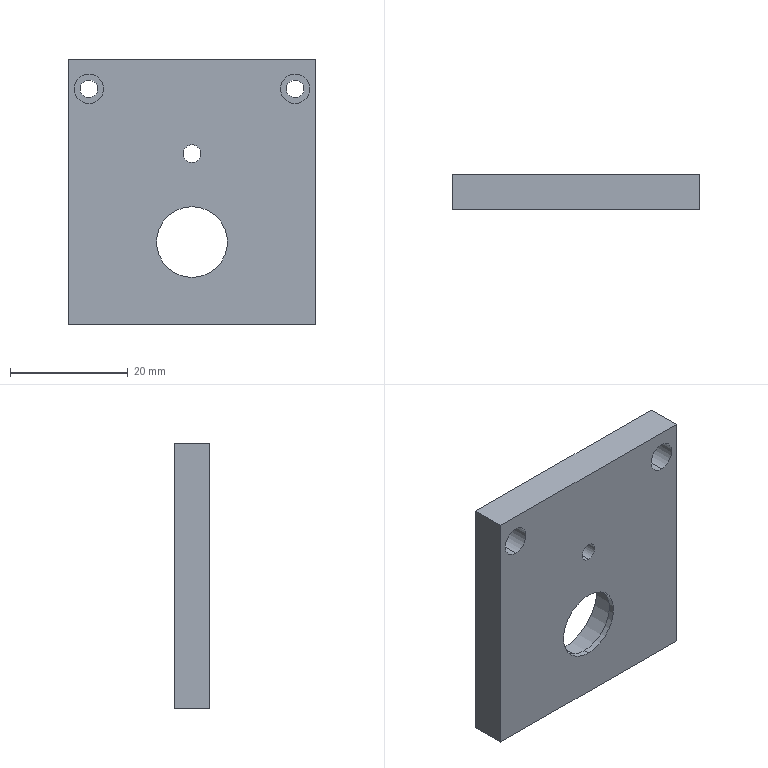Part | SolidWorks | features ICE 3, Cut 1, Extrusion 1, HoleWzd 1 | 1 solid | 31 faces | box 42 x 6 x 45 mm | volume 9918 mm3 | cylinder 18 | plane 9 | cone 4 | commonest cylinder face diameters 3 x6 2.5 x4 5 x4 12 x2 16 x2
STEP:
#1=CARTESIAN_POINT('',(13.5,3.,-5.25));
#2=VERTEX_POINT('',#1);
#3=CARTESIAN_POINT('',(13.5,3.,-7.75));
#4=VERTEX_POINT('',#3);
#5=CARTESIAN_POINT('',(13.5,3.,-6.5));
#6=DIRECTION('',(1.,0.,0.));
#7=DIRECTION('',(0.,0.,-1.));
#8=AXIS2_PLACEMENT_3D('',#5,#6,#7);
#9=CIRCLE('',#8,1.25);
#10=EDGE_CURVE('',#2,#4,#9,.T.);
#11=ORIENTED_EDGE('',*,*,#10,.F.);
#12=CARTESIAN_POINT('',(21.,3.,-5.25));
#13=VERTEX_POINT('',#12);
#14=CARTESIAN_POINT('',(21.,3.,-5.25));
#15=DIRECTION('',(1.,0.,0.));
#16=VECTOR('',#15,1000.);
#17=LINE('',#14,#16);
#18=EDGE_CURVE('',#2,#13,#17,.T.);
#19=ORIENTED_EDGE('',*,*,#18,.T.);
#20=CARTESIAN_POINT('',(21.,3.,-7.75));
#21=VERTEX_POINT('',#20);
#22=CARTESIAN_POINT('',(21.,3.,-6.5));
#23=DIRECTION('',(1.,0.,0.));
#24=DIRECTION('',(0.,0.,-1.));
#25=AXIS2_PLACEMENT_3D('',#22,#23,#24);
#26=CIRCLE('',#25,1.25);
#27=EDGE_CURVE('',#13,#21,#26,.T.);
#28=ORIENTED_EDGE('',*,*,#27,.T.);
#29=CARTESIAN_POINT('',(21.,3.,-7.75));
#30=DIRECTION('',(1.,0.,0.));
#31=VECTOR('',#30,1000.);
#32=LINE('',#29,#31);
#33=EDGE_CURVE('',#4,#21,#32,.T.);
#34=ORIENTED_EDGE('',*,*,#33,.F.);
#35=EDGE_LOOP('',(#11,#19,#28,#34));
#36=FACE_OUTER_BOUND('',#35,.T.);
#37=CARTESIAN_POINT('',(21.,3.,-6.5));
#38=DIRECTION('',(1.,0.,0.));
#39=DIRECTION('',(0.,0.,-1.));
#40=AXIS2_PLACEMENT_3D('',#37,#38,#39);
#41=CYLINDRICAL_SURFACE('',#40,1.25);
#42=ADVANCED_FACE('',(#36),#41,.F.);
#43=CARTESIAN_POINT('',(12.749,3.,-6.5));
#44=VERTEX_POINT('',#43);
#45=CARTESIAN_POINT('',(13.5,3.,-7.75));
#46=DIRECTION('',(0.515,0.,-0.8572));
#47=VECTOR('',#46,1000.);
#48=LINE('',#45,#47);
#49=EDGE_CURVE('',#44,#4,#48,.T.);
#50=ORIENTED_EDGE('',*,*,#49,.F.);
#51=CARTESIAN_POINT('',(13.5,3.,-5.25));
#52=DIRECTION('',(0.515,0.,0.8572));
#53=VECTOR('',#52,1000.);
#54=LINE('',#51,#53);
#55=EDGE_CURVE('',#44,#2,#54,.T.);
#56=ORIENTED_EDGE('',*,*,#55,.T.);
#57=ORIENTED_EDGE('',*,*,#10,.T.);
#58=EDGE_LOOP('',(#50,#56,#57));
#59=FACE_OUTER_BOUND('',#58,.T.);
#60=CARTESIAN_POINT('',(13.5,3.,-6.5));
#61=DIRECTION('',(1.,0.,0.));
#62=DIRECTION('',(0.,0.,-1.));
#63=AXIS2_PLACEMENT_3D('',#60,#61,#62);
#64=CONICAL_SURFACE('',#63,1.25,1.03);
#65=ADVANCED_FACE('',(#59),#64,.F.);
#66=CARTESIAN_POINT('',(13.5,3.,4.25));
#67=VERTEX_POINT('',#66);
#68=CARTESIAN_POINT('',(13.5,3.,1.75));
#69=VERTEX_POINT('',#68);
#70=CARTESIAN_POINT('',(13.5,3.,3.));
#71=DIRECTION('',(1.,0.,0.));
#72=DIRECTION('',(0.,0.,-1.));
#73=AXIS2_PLACEMENT_3D('',#70,#71,#72);
#74=CIRCLE('',#73,1.25);
#75=EDGE_CURVE('',#67,#69,#74,.T.);
#76=ORIENTED_EDGE('',*,*,#75,.F.);
#77=CARTESIAN_POINT('',(21.,3.,4.25));
#78=VERTEX_POINT('',#77);
#79=CARTESIAN_POINT('',(21.,3.,4.25));
#80=DIRECTION('',(1.,0.,0.));
#81=VECTOR('',#80,1000.);
#82=LINE('',#79,#81);
#83=EDGE_CURVE('',#67,#78,#82,.T.);
#84=ORIENTED_EDGE('',*,*,#83,.T.);
#85=CARTESIAN_POINT('',(21.,3.,1.75));
#86=VERTEX_POINT('',#85);
#87=CARTESIAN_POINT('',(21.,3.,3.));
#88=DIRECTION('',(1.,0.,0.));
#89=DIRECTION('',(0.,0.,-1.));
#90=AXIS2_PLACEMENT_3D('',#87,#88,#89);
#91=CIRCLE('',#90,1.25);
#92=EDGE_CURVE('',#78,#86,#91,.T.);
#93=ORIENTED_EDGE('',*,*,#92,.T.);
#94=CARTESIAN_POINT('',(21.,3.,1.75));
#95=DIRECTION('',(1.,0.,0.));
#96=VECTOR('',#95,1000.);
#97=LINE('',#94,#96);
#98=EDGE_CURVE('',#69,#86,#97,.T.);
#99=ORIENTED_EDGE('',*,*,#98,.F.);
#100=EDGE_LOOP('',(#76,#84,#93,#99));
#101=FACE_OUTER_BOUND('',#100,.T.);
#102=CARTESIAN_POINT('',(21.,3.,3.));
#103=DIRECTION('',(1.,0.,0.));
#104=DIRECTION('',(0.,0.,-1.));
#105=AXIS2_PLACEMENT_3D('',#102,#103,#104);
#106=CYLINDRICAL_SURFACE('',#105,1.25);
#107=ADVANCED_FACE('',(#101),#106,.F.);
#108=CARTESIAN_POINT('',(12.749,3.,3.));
#109=VERTEX_POINT('',#108);
#110=CARTESIAN_POINT('',(13.5,3.,1.75));
#111=DIRECTION('',(0.515,0.,-0.8572));
#112=VECTOR('',#111,1000.);
#113=LINE('',#110,#112);
#114=EDGE_CURVE('',#109,#69,#113,.T.);
#115=ORIENTED_EDGE('',*,*,#114,.F.);
#116=CARTESIAN_POINT('',(13.5,3.,4.25));
#117=DIRECTION('',(0.515,0.,0.8572));
#118=VECTOR('',#117,1000.);
#119=LINE('',#116,#118);
#120=EDGE_CURVE('',#109,#67,#119,.T.);
#121=ORIENTED_EDGE('',*,*,#120,.T.);
#122=ORIENTED_EDGE('',*,*,#75,.T.);
#123=EDGE_LOOP('',(#115,#121,#122));
#124=FACE_OUTER_BOUND('',#123,.T.);
#125=CARTESIAN_POINT('',(13.5,3.,3.));
#126=DIRECTION('',(1.,0.,0.));
#127=DIRECTION('',(0.,0.,-1.));
#128=AXIS2_PLACEMENT_3D('',#125,#126,#127);
#129=CONICAL_SURFACE('',#128,1.25,1.03);
#130=ADVANCED_FACE('',(#124),#129,.F.);
#131=CARTESIAN_POINT('',(17.5,4.,20.));
#132=VERTEX_POINT('',#131);
#133=CARTESIAN_POINT('',(17.5,4.,15.));
#134=VERTEX_POINT('',#133);
#135=CARTESIAN_POINT('',(17.5,4.,17.5));
#136=DIRECTION('',(0.,-1.,0.));
#137=DIRECTION('',(0.,0.,-1.));
#138=AXIS2_PLACEMENT_3D('',#135,#136,#137);
#139=CIRCLE('',#138,2.5);
#140=EDGE_CURVE('',#132,#134,#139,.T.);
#141=ORIENTED_EDGE('',*,*,#140,.F.);
#142=CARTESIAN_POINT('',(17.5,0.,20.));
#143=VERTEX_POINT('',#142);
#144=CARTESIAN_POINT('',(17.5,4.,20.));
#145=DIRECTION('',(0.,-1.,0.));
#146=VECTOR('',#145,1000.);
#147=LINE('',#144,#146);
#148=EDGE_CURVE('',#132,#143,#147,.T.);
#149=ORIENTED_EDGE('',*,*,#148,.T.);
#150=CARTESIAN_POINT('',(17.5,0.,15.));
#151=VERTEX_POINT('',#150);
#152=CARTESIAN_POINT('',(17.5,0.,17.5));
#153=DIRECTION('',(0.,-1.,0.));
#154=DIRECTION('',(0.,0.,-1.));
#155=AXIS2_PLACEMENT_3D('',#152,#153,#154);
#156=CIRCLE('',#155,2.5);
#157=EDGE_CURVE('',#143,#151,#156,.T.);
#158=ORIENTED_EDGE('',*,*,#157,.T.);
#159=CARTESIAN_POINT('',(17.5,4.,15.));
#160=DIRECTION('',(0.,-1.,0.));
#161=VECTOR('',#160,1000.);
#162=LINE('',#159,#161);
#163=EDGE_CURVE('',#134,#151,#162,.T.);
#164=ORIENTED_EDGE('',*,*,#163,.F.);
#165=EDGE_LOOP('',(#141,#149,#158,#164));
#166=FACE_OUTER_BOUND('',#165,.T.);
#167=CARTESIAN_POINT('',(17.5,4.,17.5));
#168=DIRECTION('',(0.,-1.,0.));
#169=DIRECTION('',(0.,0.,-1.));
#170=AXIS2_PLACEMENT_3D('',#167,#168,#169);
#171=CYLINDRICAL_SURFACE('',#170,2.5);
#172=ADVANCED_FACE('',(#166),#171,.F.);
#173=CARTESIAN_POINT('',(-17.5,4.,20.));
#174=VERTEX_POINT('',#173);
#175=CARTESIAN_POINT('',(-17.5,4.,15.));
#176=VERTEX_POINT('',#175);
#177=CARTESIAN_POINT('',(-17.5,4.,17.5));
#178=DIRECTION('',(0.,-1.,0.));
#179=DIRECTION('',(0.,0.,-1.));
#180=AXIS2_PLACEMENT_3D('',#177,#178,#179);
#181=CIRCLE('',#180,2.5);
#182=EDGE_CURVE('',#174,#176,#181,.T.);
#183=ORIENTED_EDGE('',*,*,#182,.F.);
#184=CARTESIAN_POINT('',(-17.5,0.,20.));
#185=VERTEX_POINT('',#184);
#186=CARTESIAN_POINT('',(-17.5,4.,20.));
#187=DIRECTION('',(0.,-1.,0.));
#188=VECTOR('',#187,1000.);
#189=LINE('',#186,#188);
#190=EDGE_CURVE('',#174,#185,#189,.T.);
#191=ORIENTED_EDGE('',*,*,#190,.T.);
#192=CARTESIAN_POINT('',(-17.5,0.,15.));
#193=VERTEX_POINT('',#192);
#194=CARTESIAN_POINT('',(-17.5,0.,17.5));
#195=DIRECTION('',(0.,-1.,0.));
#196=DIRECTION('',(0.,0.,-1.));
#197=AXIS2_PLACEMENT_3D('',#194,#195,#196);
#198=CIRCLE('',#197,2.5);
#199=EDGE_CURVE('',#185,#193,#198,.T.);
#200=ORIENTED_EDGE('',*,*,#199,.T.);
#201=CARTESIAN_POINT('',(-17.5,4.,15.));
#202=DIRECTION('',(0.,-1.,0.));
#203=VECTOR('',#202,1000.);
#204=LINE('',#201,#203);
#205=EDGE_CURVE('',#176,#193,#204,.T.);
#206=ORIENTED_EDGE('',*,*,#205,.F.);
#207=EDGE_LOOP('',(#183,#191,#200,#206));
#208=FACE_OUTER_BOUND('',#207,.T.);
#209=CARTESIAN_POINT('',(-17.5,4.,17.5));
#210=DIRECTION('',(0.,-1.,0.));
#211=DIRECTION('',(0.,0.,-1.));
#212=AXIS2_PLACEMENT_3D('',#209,#210,#211);
#213=CYLINDRICAL_SURFACE('',#212,2.5);
#214=ADVANCED_FACE('',(#208),#213,.F.);
#215=CARTESIAN_POINT('',(0.,1.,-16.5));
#216=VERTEX_POINT('',#215);
#217=CARTESIAN_POINT('',(0.,1.,-0.5));
#218=VERTEX_POINT('',#217);
#219=CARTESIAN_POINT('',(0.,1.,-8.5));
#220=DIRECTION('',(0.,1.,0.));
#221=DIRECTION('',(0.,0.,1.));
#222=AXIS2_PLACEMENT_3D('',#219,#220,#221);
#223=CIRCLE('',#222,8.);
#224=EDGE_CURVE('',#216,#218,#223,.T.);
#225=ORIENTED_EDGE('',*,*,#224,.F.);
#226=CARTESIAN_POINT('',(0.,6.,-16.5));
#227=VERTEX_POINT('',#226);
#228=CARTESIAN_POINT('',(0.,1.,-16.5));
#229=DIRECTION('',(0.,1.,0.));
#230=VECTOR('',#229,1000.);
#231=LINE('',#228,#230);
#232=EDGE_CURVE('',#216,#227,#231,.T.);
#233=ORIENTED_EDGE('',*,*,#232,.T.);
#234=CARTESIAN_POINT('',(0.,6.,-0.5));
#235=VERTEX_POINT('',#234);
#236=CARTESIAN_POINT('',(0.,6.,-8.5));
#237=DIRECTION('',(0.,1.,0.));
#238=DIRECTION('',(0.,0.,1.));
#239=AXIS2_PLACEMENT_3D('',#236,#237,#238);
#240=CIRCLE('',#239,8.);
#241=EDGE_CURVE('',#227,#235,#240,.T.);
#242=ORIENTED_EDGE('',*,*,#241,.T.);
#243=CARTESIAN_POINT('',(0.,1.,-0.5));
#244=DIRECTION('',(0.,1.,0.));
#245=VECTOR('',#244,1000.);
#246=LINE('',#243,#245);
#247=EDGE_CURVE('',#218,#235,#246,.T.);
#248=ORIENTED_EDGE('',*,*,#247,.F.);
#249=EDGE_LOOP('',(#225,#233,#242,#248));
#250=FACE_OUTER_BOUND('',#249,.T.);
#251=CARTESIAN_POINT('',(0.,1.,-8.5));
#252=DIRECTION('',(0.,1.,0.));
#253=DIRECTION('',(0.,0.,1.));
#254=AXIS2_PLACEMENT_3D('',#251,#252,#253);
#255=CYLINDRICAL_SURFACE('',#254,8.);
#256=ADVANCED_FACE('',(#250),#255,.F.);
#257=CARTESIAN_POINT('',(0.,6.,5.));
#258=VERTEX_POINT('',#257);
#259=CARTESIAN_POINT('',(0.,6.,8.));
#260=VERTEX_POINT('',#259);
#261=CARTESIAN_POINT('',(0.,6.,6.5));
#262=DIRECTION('',(0.,1.,0.));
#263=DIRECTION('',(0.,0.,1.));
#264=AXIS2_PLACEMENT_3D('',#261,#262,#263);
#265=CIRCLE('',#264,1.5);
#266=EDGE_CURVE('',#258,#260,#265,.T.);
#267=ORIENTED_EDGE('',*,*,#266,.T.);
#268=CARTESIAN_POINT('',(0.,0.,8.));
#269=VERTEX_POINT('',#268);
#270=CARTESIAN_POINT('',(0.,6.,8.));
#271=DIRECTION('',(0.,-1.,0.));
#272=VECTOR('',#271,1000.);
#273=LINE('',#270,#272);
#274=EDGE_CURVE('',#260,#269,#273,.T.);
#275=ORIENTED_EDGE('',*,*,#274,.T.);
#276=CARTESIAN_POINT('',(0.,0.,5.));
#277=VERTEX_POINT('',#276);
#278=CARTESIAN_POINT('',(0.,0.,6.5));
#279=DIRECTION('',(0.,1.,0.));
#280=DIRECTION('',(0.,0.,1.));
#281=AXIS2_PLACEMENT_3D('',#278,#279,#280);
#282=CIRCLE('',#281,1.5);
#283=EDGE_CURVE('',#277,#269,#282,.T.);
#284=ORIENTED_EDGE('',*,*,#283,.F.);
#285=CARTESIAN_POINT('',(0.,6.,5.));
#286=DIRECTION('',(0.,-1.,0.));
#287=VECTOR('',#286,1000.);
#288=LINE('',#285,#287);
#289=EDGE_CURVE('',#258,#277,#288,.T.);
#290=ORIENTED_EDGE('',*,*,#289,.F.);
#291=EDGE_LOOP('',(#267,#275,#284,#290));
#292=FACE_OUTER_BOUND('',#291,.T.);
#293=CARTESIAN_POINT('',(0.,6.,6.5));
#294=DIRECTION('',(0.,-1.,0.));
#295=DIRECTION('',(0.,0.,-1.));
#296=AXIS2_PLACEMENT_3D('',#293,#294,#295);
#297=CYLINDRICAL_SURFACE('',#296,1.5);
#298=ADVANCED_FACE('',(#292),#297,.F.);
#299=CARTESIAN_POINT('',(0.,1.,-14.5));
#300=VERTEX_POINT('',#299);
#301=CARTESIAN_POINT('',(0.,1.,-2.5));
#302=VERTEX_POINT('',#301);
#303=CARTESIAN_POINT('',(0.,1.,-8.5));
#304=DIRECTION('',(0.,1.,0.));
#305=DIRECTION('',(0.,0.,1.));
#306=AXIS2_PLACEMENT_3D('',#303,#304,#305);
#307=CIRCLE('',#306,6.);
#308=EDGE_CURVE('',#300,#302,#307,.T.);
#309=ORIENTED_EDGE('',*,*,#308,.T.);
#310=CARTESIAN_POINT('',(0.,0.,-2.5));
#311=VERTEX_POINT('',#310);
#312=CARTESIAN_POINT('',(0.,6.,-2.5));
#313=DIRECTION('',(0.,-1.,0.));
#314=VECTOR('',#313,1000.);
#315=LINE('',#312,#314);
#316=EDGE_CURVE('',#302,#311,#315,.T.);
#317=ORIENTED_EDGE('',*,*,#316,.T.);
#318=CARTESIAN_POINT('',(0.,0.,-14.5));
#319=VERTEX_POINT('',#318);
#320=CARTESIAN_POINT('',(0.,0.,-8.5));
#321=DIRECTION('',(0.,1.,0.));
#322=DIRECTION('',(0.,0.,1.));
#323=AXIS2_PLACEMENT_3D('',#320,#321,#322);
#324=CIRCLE('',#323,6.);
#325=EDGE_CURVE('',#319,#311,#324,.T.);
#326=ORIENTED_EDGE('',*,*,#325,.F.);
#327=CARTESIAN_POINT('',(0.,6.,-14.5));
#328=DIRECTION('',(0.,-1.,0.));
#329=VECTOR('',#328,1000.);
#330=LINE('',#327,#329);
#331=EDGE_CURVE('',#300,#319,#330,.T.);
#332=ORIENTED_EDGE('',*,*,#331,.F.);
#333=EDGE_LOOP('',(#309,#317,#326,#332));
#334=FACE_OUTER_BOUND('',#333,.T.);
#335=CARTESIAN_POINT('',(0.,6.,-8.5));
#336=DIRECTION('',(0.,-1.,0.));
#337=DIRECTION('',(0.,0.,-1.));
#338=AXIS2_PLACEMENT_3D('',#335,#336,#337);
#339=CYLINDRICAL_SURFACE('',#338,6.);
#340=ADVANCED_FACE('',(#334),#339,.F.);
#341=CARTESIAN_POINT('',(-17.5,4.,16.));
#342=VERTEX_POINT('',#341);
#343=CARTESIAN_POINT('',(-17.5,4.,19.));
#344=VERTEX_POINT('',#343);
#345=CARTESIAN_POINT('',(-17.5,4.,17.5));
#346=DIRECTION('',(0.,1.,0.));
#347=DIRECTION('',(0.,0.,-1.));
#348=AXIS2_PLACEMENT_3D('',#345,#346,#347);
#349=CIRCLE('',#348,1.5);
#350=EDGE_CURVE('',#342,#344,#349,.T.);
#351=ORIENTED_EDGE('',*,*,#350,.F.);
#352=CARTESIAN_POINT('',(-17.5,6.,16.));
#353=VERTEX_POINT('',#352);
#354=CARTESIAN_POINT('',(-17.5,0.,16.));
#355=DIRECTION('',(0.,1.,0.));
#356=VECTOR('',#355,1000.);
#357=LINE('',#354,#356);
#358=EDGE_CURVE('',#342,#353,#357,.T.);
#359=ORIENTED_EDGE('',*,*,#358,.T.);
#360=CARTESIAN_POINT('',(-17.5,6.,19.));
#361=VERTEX_POINT('',#360);
#362=CARTESIAN_POINT('',(-17.5,6.,17.5));
#363=DIRECTION('',(0.,1.,0.));
#364=DIRECTION('',(0.,0.,1.));
#365=AXIS2_PLACEMENT_3D('',#362,#363,#364);
#366=CIRCLE('',#365,1.5);
#367=EDGE_CURVE('',#353,#361,#366,.T.);
#368=ORIENTED_EDGE('',*,*,#367,.T.);
#369=CARTESIAN_POINT('',(-17.5,0.,19.));
#370=DIRECTION('',(0.,1.,0.));
#371=VECTOR('',#370,1000.);
#372=LINE('',#369,#371);
#373=EDGE_CURVE('',#344,#361,#372,.T.);
#374=ORIENTED_EDGE('',*,*,#373,.F.);
#375=EDGE_LOOP('',(#351,#359,#368,#374));
#376=FACE_OUTER_BOUND('',#375,.T.);
#377=CARTESIAN_POINT('',(-17.5,0.,17.5));
#378=DIRECTION('',(0.,1.,0.));
#379=DIRECTION('',(0.,0.,1.));
#380=AXIS2_PLACEMENT_3D('',#377,#378,#379);
#381=CYLINDRICAL_SURFACE('',#380,1.5);
#382=ADVANCED_FACE('',(#376),#381,.F.);
#383=CARTESIAN_POINT('',(17.5,4.,16.));
#384=VERTEX_POINT('',#383);
#385=CARTESIAN_POINT('',(17.5,4.,19.));
#386=VERTEX_POINT('',#385);
#387=CARTESIAN_POINT('',(17.5,4.,17.5));
#388=DIRECTION('',(0.,1.,0.));
#389=DIRECTION('',(0.,0.,-1.));
#390=AXIS2_PLACEMENT_3D('',#387,#388,#389);
#391=CIRCLE('',#390,1.5);
#392=EDGE_CURVE('',#384,#386,#391,.T.);
#393=ORIENTED_EDGE('',*,*,#392,.F.);
#394=CARTESIAN_POINT('',(17.5,6.,16.));
#395=VERTEX_POINT('',#394);
#396=CARTESIAN_POINT('',(17.5,0.,16.));
#397=DIRECTION('',(0.,1.,0.));
#398=VECTOR('',#397,1000.);
#399=LINE('',#396,#398);
#400=EDGE_CURVE('',#384,#395,#399,.T.);
#401=ORIENTED_EDGE('',*,*,#400,.T.);
#402=CARTESIAN_POINT('',(17.5,6.,19.));
#403=VERTEX_POINT('',#402);
#404=CARTESIAN_POINT('',(17.5,6.,17.5));
#405=DIRECTION('',(0.,1.,0.));
#406=DIRECTION('',(0.,0.,1.));
#407=AXIS2_PLACEMENT_3D('',#404,#405,#406);
#408=CIRCLE('',#407,1.5);
#409=EDGE_CURVE('',#395,#403,#408,.T.);
#410=ORIENTED_EDGE('',*,*,#409,.T.);
#411=CARTESIAN_POINT('',(17.5,0.,19.));
#412=DIRECTION('',(0.,1.,0.));
#413=VECTOR('',#412,1000.);
#414=LINE('',#411,#413);
#415=EDGE_CURVE('',#386,#403,#414,.T.);
#416=ORIENTED_EDGE('',*,*,#415,.F.);
#417=EDGE_LOOP('',(#393,#401,#410,#416));
#418=FACE_OUTER_BOUND('',#417,.T.);
#419=CARTESIAN_POINT('',(17.5,0.,17.5));
#420=DIRECTION('',(0.,1.,0.));
#421=DIRECTION('',(0.,0.,1.));
#422=AXIS2_PLACEMENT_3D('',#419,#420,#421);
#423=CYLINDRICAL_SURFACE('',#422,1.5);
#424=ADVANCED_FACE('',(#418),#423,.F.);
#425=ORIENTED_EDGE('',*,*,#400,.F.);
#426=CARTESIAN_POINT('',(17.5,4.,17.5));
#427=DIRECTION('',(0.,1.,0.));
#428=DIRECTION('',(0.,0.,-1.));
#429=AXIS2_PLACEMENT_3D('',#426,#427,#428);
#430=CIRCLE('',#429,1.5);
#431=EDGE_CURVE('',#386,#384,#430,.T.);
#432=ORIENTED_EDGE('',*,*,#431,.F.);
#433=ORIENTED_EDGE('',*,*,#415,.T.);
#434=CARTESIAN_POINT('',(17.5,6.,17.5));
#435=DIRECTION('',(0.,1.,0.));
#436=DIRECTION('',(0.,0.,1.));
#437=AXIS2_PLACEMENT_3D('',#434,#435,#436);
#438=CIRCLE('',#437,1.5);
#439=EDGE_CURVE('',#403,#395,#438,.T.);
#440=ORIENTED_EDGE('',*,*,#439,.T.);
#441=EDGE_LOOP('',(#425,#432,#433,#440));
#442=FACE_OUTER_BOUND('',#441,.T.);
#443=CARTESIAN_POINT('',(17.5,0.,17.5));
#444=DIRECTION('',(0.,1.,0.));
#445=DIRECTION('',(0.,0.,1.));
#446=AXIS2_PLACEMENT_3D('',#443,#444,#445);
#447=CYLINDRICAL_SURFACE('',#446,1.5);
#448=ADVANCED_FACE('',(#442),#447,.F.);
#449=ORIENTED_EDGE('',*,*,#358,.F.);
#450=CARTESIAN_POINT('',(-17.5,4.,17.5));
#451=DIRECTION('',(0.,1.,0.));
#452=DIRECTION('',(0.,0.,-1.));
#453=AXIS2_PLACEMENT_3D('',#450,#451,#452);
#454=CIRCLE('',#453,1.5);
#455=EDGE_CURVE('',#344,#342,#454,.T.);
#456=ORIENTED_EDGE('',*,*,#455,.F.);
#457=ORIENTED_EDGE('',*,*,#373,.T.);
#458=CARTESIAN_POINT('',(-17.5,6.,17.5));
#459=DIRECTION('',(0.,1.,0.));
#460=DIRECTION('',(0.,0.,1.));
#461=AXIS2_PLACEMENT_3D('',#458,#459,#460);
#462=CIRCLE('',#461,1.5);
#463=EDGE_CURVE('',#361,#353,#462,.T.);
#464=ORIENTED_EDGE('',*,*,#463,.T.);
#465=EDGE_LOOP('',(#449,#456,#457,#464));
#466=FACE_OUTER_BOUND('',#465,.T.);
#467=CARTESIAN_POINT('',(-17.5,0.,17.5));
#468=DIRECTION('',(0.,1.,0.));
#469=DIRECTION('',(0.,0.,1.));
#470=AXIS2_PLACEMENT_3D('',#467,#468,#469);
#471=CYLINDRICAL_SURFACE('',#470,1.5);
#472=ADVANCED_FACE('',(#466),#471,.F.);
#473=ORIENTED_EDGE('',*,*,#316,.F.);
#474=CARTESIAN_POINT('',(0.,1.,-8.5));
#475=DIRECTION('',(0.,1.,0.));
#476=DIRECTION('',(0.,0.,1.));
#477=AXIS2_PLACEMENT_3D('',#474,#475,#476);
#478=CIRCLE('',#477,6.);
#479=EDGE_CURVE('',#302,#300,#478,.T.);
#480=ORIENTED_EDGE('',*,*,#479,.T.);
#481=ORIENTED_EDGE('',*,*,#331,.T.);
#482=CARTESIAN_POINT('',(0.,0.,-8.5));
#483=DIRECTION('',(0.,1.,0.));
#484=DIRECTION('',(0.,0.,1.));
#485=AXIS2_PLACEMENT_3D('',#482,#483,#484);
#486=CIRCLE('',#485,6.);
#487=EDGE_CURVE('',#311,#319,#486,.T.);
#488=ORIENTED_EDGE('',*,*,#487,.F.);
#489=EDGE_LOOP('',(#473,#480,#481,#488));
#490=FACE_OUTER_BOUND('',#489,.T.);
#491=CARTESIAN_POINT('',(0.,6.,-8.5));
#492=DIRECTION('',(0.,-1.,0.));
#493=DIRECTION('',(0.,0.,-1.));
#494=AXIS2_PLACEMENT_3D('',#491,#492,#493);
#495=CYLINDRICAL_SURFACE('',#494,6.);
#496=ADVANCED_FACE('',(#490),#495,.F.);
#497=ORIENTED_EDGE('',*,*,#463,.F.);
#498=ORIENTED_EDGE('',*,*,#367,.F.);
#499=EDGE_LOOP('',(#497,#498));
#500=FACE_BOUND('',#499,.T.);
#501=ORIENTED_EDGE('',*,*,#439,.F.);
#502=ORIENTED_EDGE('',*,*,#409,.F.);
#503=EDGE_LOOP('',(#501,#502));
#504=FACE_BOUND('',#503,.T.);
#505=CARTESIAN_POINT('',(0.,6.,-8.5));
#506=DIRECTION('',(0.,1.,0.));
#507=DIRECTION('',(0.,0.,1.));
#508=AXIS2_PLACEMENT_3D('',#505,#506,#507);
#509=CIRCLE('',#508,8.);
#510=EDGE_CURVE('',#235,#227,#509,.T.);
#511=ORIENTED_EDGE('',*,*,#510,.F.);
#512=ORIENTED_EDGE('',*,*,#241,.F.);
#513=EDGE_LOOP('',(#511,#512));
#514=FACE_BOUND('',#513,.T.);
#515=CARTESIAN_POINT('',(21.,6.,22.5));
#516=VERTEX_POINT('',#515);
#517=CARTESIAN_POINT('',(21.,6.,-22.5));
#518=VERTEX_POINT('',#517);
#519=CARTESIAN_POINT('',(21.,6.,-22.5));
#520=DIRECTION('',(0.,0.,-1.));
#521=VECTOR('',#520,1000.);
#522=LINE('',#519,#521);
#523=EDGE_CURVE('',#516,#518,#522,.T.);
#524=ORIENTED_EDGE('',*,*,#523,.T.);
#525=CARTESIAN_POINT('',(-21.,6.,-22.5));
#526=VERTEX_POINT('',#525);
#527=CARTESIAN_POINT('',(-21.,6.,-22.5));
#528=DIRECTION('',(-1.,0.,0.));
#529=VECTOR('',#528,1000.);
#530=LINE('',#527,#529);
#531=EDGE_CURVE('',#518,#526,#530,.T.);
#532=ORIENTED_EDGE('',*,*,#531,.T.);
#533=CARTESIAN_POINT('',(-21.,6.,22.5));
#534=VERTEX_POINT('',#533);
#535=CARTESIAN_POINT('',(-21.,6.,-22.5));
#536=DIRECTION('',(0.,0.,1.));
#537=VECTOR('',#536,1000.);
#538=LINE('',#535,#537);
#539=EDGE_CURVE('',#526,#534,#538,.T.);
#540=ORIENTED_EDGE('',*,*,#539,.T.);
#541=CARTESIAN_POINT('',(-21.,6.,22.5));
#542=DIRECTION('',(1.,0.,0.));
#543=VECTOR('',#542,1000.);
#544=LINE('',#541,#543);
#545=EDGE_CURVE('',#534,#516,#544,.T.);
#546=ORIENTED_EDGE('',*,*,#545,.T.);
#547=EDGE_LOOP('',(#524,#532,#540,#546));
#548=FACE_OUTER_BOUND('',#547,.T.);
#549=ORIENTED_EDGE('',*,*,#266,.F.);
#550=CARTESIAN_POINT('',(0.,6.,6.5));
#551=DIRECTION('',(0.,1.,0.));
#552=DIRECTION('',(0.,0.,1.));
#553=AXIS2_PLACEMENT_3D('',#550,#551,#552);
#554=CIRCLE('',#553,1.5);
#555=EDGE_CURVE('',#260,#258,#554,.T.);
#556=ORIENTED_EDGE('',*,*,#555,.F.);
#557=EDGE_LOOP('',(#549,#556));
#558=FACE_BOUND('',#557,.T.);
#559=CARTESIAN_POINT('',(0.,6.,0.));
#560=DIRECTION('',(0.,1.,0.));
#561=DIRECTION('',(0.,0.,1.));
#562=AXIS2_PLACEMENT_3D('',#559,#560,#561);
#563=PLANE('',#562);
#564=ADVANCED_FACE('',(#500,#504,#514,#548,#558),#563,.T.);
#565=CARTESIAN_POINT('',(17.5,0.,17.5));
#566=DIRECTION('',(0.,-1.,0.));
#567=DIRECTION('',(0.,0.,-1.));
#568=AXIS2_PLACEMENT_3D('',#565,#566,#567);
#569=CIRCLE('',#568,2.5);
#570=EDGE_CURVE('',#151,#143,#569,.T.);
#571=ORIENTED_EDGE('',*,*,#570,.F.);
#572=ORIENTED_EDGE('',*,*,#157,.F.);
#573=EDGE_LOOP('',(#571,#572));
#574=FACE_BOUND('',#573,.T.);
#575=CARTESIAN_POINT('',(-17.5,0.,17.5));
#576=DIRECTION('',(0.,-1.,0.));
#577=DIRECTION('',(0.,0.,-1.));
#578=AXIS2_PLACEMENT_3D('',#575,#576,#577);
#579=CIRCLE('',#578,2.5);
#580=EDGE_CURVE('',#193,#185,#579,.T.);
#581=ORIENTED_EDGE('',*,*,#580,.F.);
#582=ORIENTED_EDGE('',*,*,#199,.F.);
#583=EDGE_LOOP('',(#581,#582));
#584=FACE_BOUND('',#583,.T.);
#585=CARTESIAN_POINT('',(21.,0.,22.5));
#586=VERTEX_POINT('',#585);
#587=CARTESIAN_POINT('',(21.,0.,-22.5));
#588=VERTEX_POINT('',#587);
#589=CARTESIAN_POINT('',(21.,0.,-22.5));
#590=DIRECTION('',(0.,0.,-1.));
#591=VECTOR('',#590,1000.);
#592=LINE('',#589,#591);
#593=EDGE_CURVE('',#586,#588,#592,.T.);
#594=ORIENTED_EDGE('',*,*,#593,.F.);
#595=CARTESIAN_POINT('',(-21.,0.,22.5));
#596=VERTEX_POINT('',#595);
#597=CARTESIAN_POINT('',(-21.,0.,22.5));
#598=DIRECTION('',(1.,0.,0.));
#599=VECTOR('',#598,1000.);
#600=LINE('',#597,#599);
#601=EDGE_CURVE('',#596,#586,#600,.T.);
#602=ORIENTED_EDGE('',*,*,#601,.F.);
#603=CARTESIAN_POINT('',(-21.,0.,-22.5));
#604=VERTEX_POINT('',#603);
#605=CARTESIAN_POINT('',(-21.,0.,-22.5));
#606=DIRECTION('',(0.,0.,1.));
#607=VECTOR('',#606,1000.);
#608=LINE('',#605,#607);
#609=EDGE_CURVE('',#604,#596,#608,.T.);
#610=ORIENTED_EDGE('',*,*,#609,.F.);
#611=CARTESIAN_POINT('',(-21.,0.,-22.5));
#612=DIRECTION('',(-1.,0.,0.));
#613=VECTOR('',#612,1000.);
#614=LINE('',#611,#613);
#615=EDGE_CURVE('',#588,#604,#614,.T.);
#616=ORIENTED_EDGE('',*,*,#615,.F.);
#617=EDGE_LOOP('',(#594,#602,#610,#616));
#618=FACE_OUTER_BOUND('',#617,.T.);
#619=ORIENTED_EDGE('',*,*,#325,.T.);
#620=ORIENTED_EDGE('',*,*,#487,.T.);
#621=EDGE_LOOP('',(#619,#620));
#622=FACE_BOUND('',#621,.T.);
#623=ORIENTED_EDGE('',*,*,#283,.T.);
#624=CARTESIAN_POINT('',(0.,0.,6.5));
#625=DIRECTION('',(0.,1.,0.));
#626=DIRECTION('',(0.,0.,1.));
#627=AXIS2_PLACEMENT_3D('',#624,#625,#626);
#628=CIRCLE('',#627,1.5);
#629=EDGE_CURVE('',#269,#277,#628,.T.);
#630=ORIENTED_EDGE('',*,*,#629,.T.);
#631=EDGE_LOOP('',(#623,#630));
#632=FACE_BOUND('',#631,.T.);
#633=CARTESIAN_POINT('',(0.,0.,0.));
#634=DIRECTION('',(0.,1.,0.));
#635=DIRECTION('',(0.,0.,1.));
#636=AXIS2_PLACEMENT_3D('',#633,#634,#635);
#637=PLANE('',#636);
#638=ADVANCED_FACE('',(#574,#584,#618,#622,#632),#637,.F.);
#639=CARTESIAN_POINT('',(21.,3.,-6.5));
#640=DIRECTION('',(1.,0.,0.));
#641=DIRECTION('',(0.,0.,-1.));
#642=AXIS2_PLACEMENT_3D('',#639,#640,#641);
#643=CIRCLE('',#642,1.25);
#644=EDGE_CURVE('',#21,#13,#643,.T.);
#645=ORIENTED_EDGE('',*,*,#644,.F.);
#646=ORIENTED_EDGE('',*,*,#27,.F.);
#647=EDGE_LOOP('',(#645,#646));
#648=FACE_BOUND('',#647,.T.);
#649=CARTESIAN_POINT('',(21.,3.,3.));
#650=DIRECTION('',(1.,0.,0.));
#651=DIRECTION('',(0.,0.,-1.));
#652=AXIS2_PLACEMENT_3D('',#649,#650,#651);
#653=CIRCLE('',#652,1.25);
#654=EDGE_CURVE('',#86,#78,#653,.T.);
#655=ORIENTED_EDGE('',*,*,#654,.F.);
#656=ORIENTED_EDGE('',*,*,#92,.F.);
#657=EDGE_LOOP('',(#655,#656));
#658=FACE_BOUND('',#657,.T.);
#659=ORIENTED_EDGE('',*,*,#593,.T.);
#660=CARTESIAN_POINT('',(21.,6.,-22.5));
#661=DIRECTION('',(0.,-1.,0.));
#662=VECTOR('',#661,1000.);
#663=LINE('',#660,#662);
#664=EDGE_CURVE('',#518,#588,#663,.T.);
#665=ORIENTED_EDGE('',*,*,#664,.F.);
#666=ORIENTED_EDGE('',*,*,#523,.F.);
#667=CARTESIAN_POINT('',(21.,6.,22.5));
#668=DIRECTION('',(0.,-1.,0.));
#669=VECTOR('',#668,1000.);
#670=LINE('',#667,#669);
#671=EDGE_CURVE('',#516,#586,#670,.T.);
#672=ORIENTED_EDGE('',*,*,#671,.T.);
#673=EDGE_LOOP('',(#659,#665,#666,#672));
#674=FACE_OUTER_BOUND('',#673,.T.);
#675=CARTESIAN_POINT('',(21.,6.,-22.5));
#676=DIRECTION('',(-1.,0.,0.));
#677=DIRECTION('',(0.,0.,1.));
#678=AXIS2_PLACEMENT_3D('',#675,#676,#677);
#679=PLANE('',#678);
#680=ADVANCED_FACE('',(#648,#658,#674),#679,.F.);
#681=ORIENTED_EDGE('',*,*,#615,.T.);
#682=CARTESIAN_POINT('',(-21.,6.,-22.5));
#683=DIRECTION('',(0.,-1.,0.));
#684=VECTOR('',#683,1000.);
#685=LINE('',#682,#684);
#686=EDGE_CURVE('',#526,#604,#685,.T.);
#687=ORIENTED_EDGE('',*,*,#686,.F.);
#688=ORIENTED_EDGE('',*,*,#531,.F.);
#689=ORIENTED_EDGE('',*,*,#664,.T.);
#690=EDGE_LOOP('',(#681,#687,#688,#689));
#691=FACE_OUTER_BOUND('',#690,.T.);
#692=CARTESIAN_POINT('',(-21.,6.,-22.5));
#693=DIRECTION('',(0.,0.,1.));
#694=DIRECTION('',(1.,0.,0.));
#695=AXIS2_PLACEMENT_3D('',#692,#693,#694);
#696=PLANE('',#695);
#697=ADVANCED_FACE('',(#691),#696,.F.);
#698=ORIENTED_EDGE('',*,*,#609,.T.);
#699=CARTESIAN_POINT('',(-21.,6.,22.5));
#700=DIRECTION('',(0.,-1.,0.));
#701=VECTOR('',#700,1000.);
#702=LINE('',#699,#701);
#703=EDGE_CURVE('',#534,#596,#702,.T.);
#704=ORIENTED_EDGE('',*,*,#703,.F.);
#705=ORIENTED_EDGE('',*,*,#539,.F.);
#706=ORIENTED_EDGE('',*,*,#686,.T.);
#707=EDGE_LOOP('',(#698,#704,#705,#706));
#708=FACE_OUTER_BOUND('',#707,.T.);
#709=CARTESIAN_POINT('',(-21.,6.,-22.5));
#710=DIRECTION('',(1.,0.,0.));
#711=DIRECTION('',(0.,0.,-1.));
#712=AXIS2_PLACEMENT_3D('',#709,#710,#711);
#713=PLANE('',#712);
#714=ADVANCED_FACE('',(#708),#713,.F.);
#715=ORIENTED_EDGE('',*,*,#601,.T.);
#716=ORIENTED_EDGE('',*,*,#671,.F.);
#717=ORIENTED_EDGE('',*,*,#545,.F.);
#718=ORIENTED_EDGE('',*,*,#703,.T.);
#719=EDGE_LOOP('',(#715,#716,#717,#718));
#720=FACE_OUTER_BOUND('',#719,.T.);
#721=CARTESIAN_POINT('',(-21.,6.,22.5));
#722=DIRECTION('',(0.,0.,-1.));
#723=DIRECTION('',(-1.,0.,0.));
#724=AXIS2_PLACEMENT_3D('',#721,#722,#723);
#725=PLANE('',#724);
#726=ADVANCED_FACE('',(#720),#725,.F.);
#727=ORIENTED_EDGE('',*,*,#274,.F.);
#728=ORIENTED_EDGE('',*,*,#555,.T.);
#729=ORIENTED_EDGE('',*,*,#289,.T.);
#730=ORIENTED_EDGE('',*,*,#629,.F.);
#731=EDGE_LOOP('',(#727,#728,#729,#730));
#732=FACE_OUTER_BOUND('',#731,.T.);
#733=CARTESIAN_POINT('',(0.,6.,6.5));
#734=DIRECTION('',(0.,-1.,0.));
#735=DIRECTION('',(0.,0.,-1.));
#736=AXIS2_PLACEMENT_3D('',#733,#734,#735);
#737=CYLINDRICAL_SURFACE('',#736,1.5);
#738=ADVANCED_FACE('',(#732),#737,.F.);
#739=ORIENTED_EDGE('',*,*,#232,.F.);
#740=CARTESIAN_POINT('',(0.,1.,-8.5));
#741=DIRECTION('',(0.,1.,0.));
#742=DIRECTION('',(0.,0.,1.));
#743=AXIS2_PLACEMENT_3D('',#740,#741,#742);
#744=CIRCLE('',#743,8.);
#745=EDGE_CURVE('',#218,#216,#744,.T.);
#746=ORIENTED_EDGE('',*,*,#745,.F.);
#747=ORIENTED_EDGE('',*,*,#247,.T.);
#748=ORIENTED_EDGE('',*,*,#510,.T.);
#749=EDGE_LOOP('',(#739,#746,#747,#748));
#750=FACE_OUTER_BOUND('',#749,.T.);
#751=CARTESIAN_POINT('',(0.,1.,-8.5));
#752=DIRECTION('',(0.,1.,0.));
#753=DIRECTION('',(0.,0.,1.));
#754=AXIS2_PLACEMENT_3D('',#751,#752,#753);
#755=CYLINDRICAL_SURFACE('',#754,8.);
#756=ADVANCED_FACE('',(#750),#755,.F.);
#757=ORIENTED_EDGE('',*,*,#308,.F.);
#758=ORIENTED_EDGE('',*,*,#479,.F.);
#759=EDGE_LOOP('',(#757,#758));
#760=FACE_BOUND('',#759,.T.);
#761=ORIENTED_EDGE('',*,*,#745,.T.);
#762=ORIENTED_EDGE('',*,*,#224,.T.);
#763=EDGE_LOOP('',(#761,#762));
#764=FACE_OUTER_BOUND('',#763,.T.);
#765=CARTESIAN_POINT('',(0.,1.,-8.5));
#766=DIRECTION('',(0.,1.,0.));
#767=DIRECTION('',(0.,0.,1.));
#768=AXIS2_PLACEMENT_3D('',#765,#766,#767);
#769=PLANE('',#768);
#770=ADVANCED_FACE('',(#760,#764),#769,.T.);
#771=CARTESIAN_POINT('',(-17.5,4.,17.5));
#772=DIRECTION('',(0.,-1.,0.));
#773=DIRECTION('',(0.,0.,-1.));
#774=AXIS2_PLACEMENT_3D('',#771,#772,#773);
#775=CIRCLE('',#774,2.5);
#776=EDGE_CURVE('',#176,#174,#775,.T.);
#777=ORIENTED_EDGE('',*,*,#776,.T.);
#778=ORIENTED_EDGE('',*,*,#182,.T.);
#779=EDGE_LOOP('',(#777,#778));
#780=FACE_OUTER_BOUND('',#779,.T.);
#781=ORIENTED_EDGE('',*,*,#455,.T.);
#782=ORIENTED_EDGE('',*,*,#350,.T.);
#783=EDGE_LOOP('',(#781,#782));
#784=FACE_BOUND('',#783,.T.);
#785=CARTESIAN_POINT('',(-17.5,4.,17.5));
#786=DIRECTION('',(0.,-1.,0.));
#787=DIRECTION('',(0.,0.,-1.));
#788=AXIS2_PLACEMENT_3D('',#785,#786,#787);
#789=PLANE('',#788);
#790=ADVANCED_FACE('',(#780,#784),#789,.T.);
#791=ORIENTED_EDGE('',*,*,#190,.F.);
#792=ORIENTED_EDGE('',*,*,#776,.F.);
#793=ORIENTED_EDGE('',*,*,#205,.T.);
#794=ORIENTED_EDGE('',*,*,#580,.T.);
#795=EDGE_LOOP('',(#791,#792,#793,#794));
#796=FACE_OUTER_BOUND('',#795,.T.);
#797=CARTESIAN_POINT('',(-17.5,4.,17.5));
#798=DIRECTION('',(0.,-1.,0.));
#799=DIRECTION('',(0.,0.,-1.));
#800=AXIS2_PLACEMENT_3D('',#797,#798,#799);
#801=CYLINDRICAL_SURFACE('',#800,2.5);
#802=ADVANCED_FACE('',(#796),#801,.F.);
#803=CARTESIAN_POINT('',(17.5,4.,17.5));
#804=DIRECTION('',(0.,-1.,0.));
#805=DIRECTION('',(0.,0.,-1.));
#806=AXIS2_PLACEMENT_3D('',#803,#804,#805);
#807=CIRCLE('',#806,2.5);
#808=EDGE_CURVE('',#134,#132,#807,.T.);
#809=ORIENTED_EDGE('',*,*,#808,.T.);
#810=ORIENTED_EDGE('',*,*,#140,.T.);
#811=EDGE_LOOP('',(#809,#810));
#812=FACE_OUTER_BOUND('',#811,.T.);
#813=ORIENTED_EDGE('',*,*,#431,.T.);
#814=ORIENTED_EDGE('',*,*,#392,.T.);
#815=EDGE_LOOP('',(#813,#814));
#816=FACE_BOUND('',#815,.T.);
#817=CARTESIAN_POINT('',(17.5,4.,17.5));
#818=DIRECTION('',(0.,-1.,0.));
#819=DIRECTION('',(0.,0.,-1.));
#820=AXIS2_PLACEMENT_3D('',#817,#818,#819);
#821=PLANE('',#820);
#822=ADVANCED_FACE('',(#812,#816),#821,.T.);
#823=ORIENTED_EDGE('',*,*,#148,.F.);
#824=ORIENTED_EDGE('',*,*,#808,.F.);
#825=ORIENTED_EDGE('',*,*,#163,.T.);
#826=ORIENTED_EDGE('',*,*,#570,.T.);
#827=EDGE_LOOP('',(#823,#824,#825,#826));
#828=FACE_OUTER_BOUND('',#827,.T.);
#829=CARTESIAN_POINT('',(17.5,4.,17.5));
#830=DIRECTION('',(0.,-1.,0.));
#831=DIRECTION('',(0.,0.,-1.));
#832=AXIS2_PLACEMENT_3D('',#829,#830,#831);
#833=CYLINDRICAL_SURFACE('',#832,2.5);
#834=ADVANCED_FACE('',(#828),#833,.F.);
#835=ORIENTED_EDGE('',*,*,#120,.F.);
#836=ORIENTED_EDGE('',*,*,#114,.T.);
#837=CARTESIAN_POINT('',(13.5,3.,3.));
#838=DIRECTION('',(1.,0.,0.));
#839=DIRECTION('',(0.,0.,-1.));
#840=AXIS2_PLACEMENT_3D('',#837,#838,#839);
#841=CIRCLE('',#840,1.25);
#842=EDGE_CURVE('',#69,#67,#841,.T.);
#843=ORIENTED_EDGE('',*,*,#842,.T.);
#844=EDGE_LOOP('',(#835,#836,#843));
#845=FACE_OUTER_BOUND('',#844,.T.);
#846=CARTESIAN_POINT('',(13.5,3.,3.));
#847=DIRECTION('',(1.,0.,0.));
#848=DIRECTION('',(0.,0.,-1.));
#849=AXIS2_PLACEMENT_3D('',#846,#847,#848);
#850=CONICAL_SURFACE('',#849,1.25,1.03);
#851=ADVANCED_FACE('',(#845),#850,.F.);
#852=ORIENTED_EDGE('',*,*,#83,.F.);
#853=ORIENTED_EDGE('',*,*,#842,.F.);
#854=ORIENTED_EDGE('',*,*,#98,.T.);
#855=ORIENTED_EDGE('',*,*,#654,.T.);
#856=EDGE_LOOP('',(#852,#853,#854,#855));
#857=FACE_OUTER_BOUND('',#856,.T.);
#858=CARTESIAN_POINT('',(21.,3.,3.));
#859=DIRECTION('',(1.,0.,0.));
#860=DIRECTION('',(0.,0.,-1.));
#861=AXIS2_PLACEMENT_3D('',#858,#859,#860);
#862=CYLINDRICAL_SURFACE('',#861,1.25);
#863=ADVANCED_FACE('',(#857),#862,.F.);
#864=ORIENTED_EDGE('',*,*,#55,.F.);
#865=ORIENTED_EDGE('',*,*,#49,.T.);
#866=CARTESIAN_POINT('',(13.5,3.,-6.5));
#867=DIRECTION('',(1.,0.,0.));
#868=DIRECTION('',(0.,0.,-1.));
#869=AXIS2_PLACEMENT_3D('',#866,#867,#868);
#870=CIRCLE('',#869,1.25);
#871=EDGE_CURVE('',#4,#2,#870,.T.);
#872=ORIENTED_EDGE('',*,*,#871,.T.);
#873=EDGE_LOOP('',(#864,#865,#872));
#874=FACE_OUTER_BOUND('',#873,.T.);
#875=CARTESIAN_POINT('',(13.5,3.,-6.5));
#876=DIRECTION('',(1.,0.,0.));
#877=DIRECTION('',(0.,0.,-1.));
#878=AXIS2_PLACEMENT_3D('',#875,#876,#877);
#879=CONICAL_SURFACE('',#878,1.25,1.03);
#880=ADVANCED_FACE('',(#874),#879,.F.);
#881=ORIENTED_EDGE('',*,*,#18,.F.);
#882=ORIENTED_EDGE('',*,*,#871,.F.);
#883=ORIENTED_EDGE('',*,*,#33,.T.);
#884=ORIENTED_EDGE('',*,*,#644,.T.);
#885=EDGE_LOOP('',(#881,#882,#883,#884));
#886=FACE_OUTER_BOUND('',#885,.T.);
#887=CARTESIAN_POINT('',(21.,3.,-6.5));
#888=DIRECTION('',(1.,0.,0.));
#889=DIRECTION('',(0.,0.,-1.));
#890=AXIS2_PLACEMENT_3D('',#887,#888,#889);
#891=CYLINDRICAL_SURFACE('',#890,1.25);
#892=ADVANCED_FACE('',(#886),#891,.F.);
#893=CLOSED_SHELL('',(#42,#65,#107,#130,#172,#214,#256,#298,#340,#382,#424,#448,#472,#496,#564,#638,#680,#697,#714,#726,#738,#756,#770,#790,#802,#822,#834,#851,#863,#880,#892));
#894=MANIFOLD_SOLID_BREP('',#893);
#895=CARTESIAN_POINT('',(0.,0.,0.));
#896=DIRECTION('',(0.,0.,1.));
#897=DIRECTION('',(1.,0.,0.));
#898=AXIS2_PLACEMENT_3D('',#895,#896,#897);
#899=(LENGTH_UNIT()NAMED_UNIT(*)SI_UNIT(.MILLI.,.METRE.));
#900=UNCERTAINTY_MEASURE_WITH_UNIT(LENGTH_MEASURE(0.00001),#899,'','');
#901=(NAMED_UNIT(*)PLANE_ANGLE_UNIT()SI_UNIT($,.RADIAN.));
#902=(NAMED_UNIT(*)SI_UNIT($,.STERADIAN.)SOLID_ANGLE_UNIT());
#903=(GEOMETRIC_REPRESENTATION_CONTEXT(3)GLOBAL_UNCERTAINTY_ASSIGNED_CONTEXT((#900))GLOBAL_UNIT_ASSIGNED_CONTEXT((#899,#901,#902))REPRESENTATION_CONTEXT('',''));
#904=ADVANCED_BREP_SHAPE_REPRESENTATION('',(#894,#898),#903);